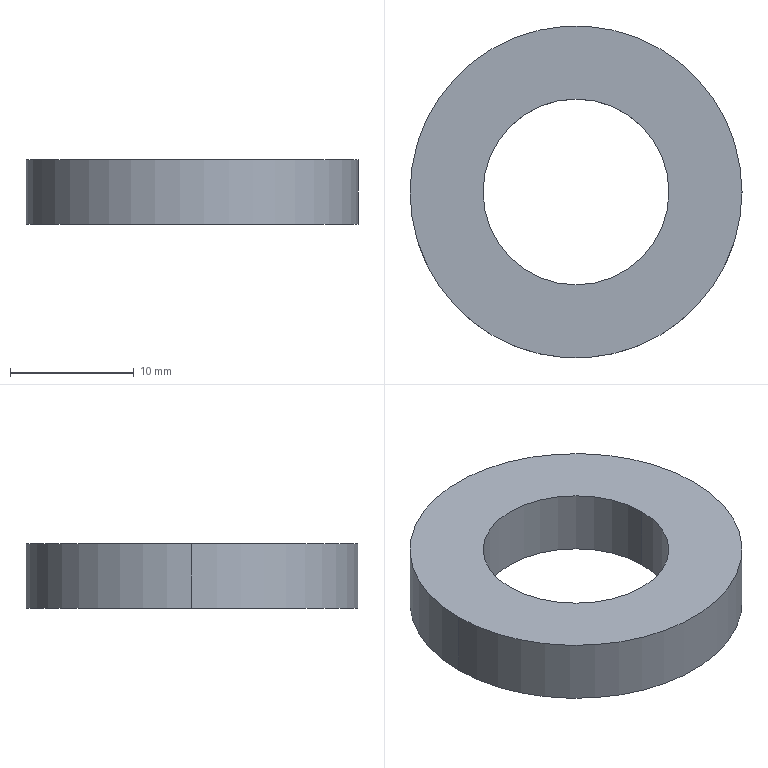Part | SolidWorks | features BaseBody 1 | 1 solid | 6 faces | box 26.799 x 26.799 x 5.237 mm | volume 2029 mm3 | cylinder 4 | plane 2 | commonest cylinder face diameters 15 x2 26.799 x2
STEP:
#1=CARTESIAN_POINT('',(17.927,0.,0.));
#2=VERTEX_POINT('',#1);
#3=CARTESIAN_POINT('',(-8.872,0.,0.));
#4=VERTEX_POINT('',#3);
#5=CARTESIAN_POINT('',(4.528,0.,0.));
#6=DIRECTION('',(0.,0.,1.));
#7=DIRECTION('',(1.,0.,0.));
#8=AXIS2_PLACEMENT_3D('',#5,#6,#7);
#9=CIRCLE('',#8,13.4);
#10=EDGE_CURVE('',#2,#4,#9,.T.);
#11=ORIENTED_EDGE('',*,*,#10,.T.);
#12=CARTESIAN_POINT('',(-8.872,0.,5.237));
#13=VERTEX_POINT('',#12);
#14=CARTESIAN_POINT('',(-8.872,0.,0.));
#15=DIRECTION('',(0.,0.,1.));
#16=VECTOR('',#15,1000.);
#17=LINE('',#14,#16);
#18=EDGE_CURVE('',#4,#13,#17,.T.);
#19=ORIENTED_EDGE('',*,*,#18,.T.);
#20=CARTESIAN_POINT('',(17.927,0.,5.237));
#21=VERTEX_POINT('',#20);
#22=CARTESIAN_POINT('',(4.528,0.,5.237));
#23=DIRECTION('',(0.,0.,-1.));
#24=DIRECTION('',(1.,0.,0.));
#25=AXIS2_PLACEMENT_3D('',#22,#23,#24);
#26=CIRCLE('',#25,13.4);
#27=EDGE_CURVE('',#13,#21,#26,.T.);
#28=ORIENTED_EDGE('',*,*,#27,.T.);
#29=CARTESIAN_POINT('',(17.927,0.,0.));
#30=DIRECTION('',(0.,0.,1.));
#31=VECTOR('',#30,1000.);
#32=LINE('',#29,#31);
#33=EDGE_CURVE('',#2,#21,#32,.T.);
#34=ORIENTED_EDGE('',*,*,#33,.F.);
#35=EDGE_LOOP('',(#11,#19,#28,#34));
#36=FACE_OUTER_BOUND('',#35,.T.);
#37=CARTESIAN_POINT('',(4.528,0.,0.));
#38=DIRECTION('',(0.,0.,1.));
#39=DIRECTION('',(1.,0.,0.));
#40=AXIS2_PLACEMENT_3D('',#37,#38,#39);
#41=CYLINDRICAL_SURFACE('',#40,13.4);
#42=ADVANCED_FACE('',(#36),#41,.T.);
#43=CARTESIAN_POINT('',(12.028,0.,0.));
#44=VERTEX_POINT('',#43);
#45=CARTESIAN_POINT('',(-2.972,0.,0.));
#46=VERTEX_POINT('',#45);
#47=CARTESIAN_POINT('',(4.528,0.,0.));
#48=DIRECTION('',(0.,0.,-1.));
#49=DIRECTION('',(1.,0.,0.));
#50=AXIS2_PLACEMENT_3D('',#47,#48,#49);
#51=CIRCLE('',#50,7.5);
#52=EDGE_CURVE('',#44,#46,#51,.T.);
#53=ORIENTED_EDGE('',*,*,#52,.T.);
#54=CARTESIAN_POINT('',(-2.972,0.,5.237));
#55=VERTEX_POINT('',#54);
#56=CARTESIAN_POINT('',(-2.972,0.,0.));
#57=DIRECTION('',(0.,0.,1.));
#58=VECTOR('',#57,1000.);
#59=LINE('',#56,#58);
#60=EDGE_CURVE('',#46,#55,#59,.T.);
#61=ORIENTED_EDGE('',*,*,#60,.T.);
#62=CARTESIAN_POINT('',(12.028,0.,5.237));
#63=VERTEX_POINT('',#62);
#64=CARTESIAN_POINT('',(4.528,0.,5.237));
#65=DIRECTION('',(0.,0.,-1.));
#66=DIRECTION('',(1.,0.,0.));
#67=AXIS2_PLACEMENT_3D('',#64,#65,#66);
#68=CIRCLE('',#67,7.5);
#69=EDGE_CURVE('',#63,#55,#68,.T.);
#70=ORIENTED_EDGE('',*,*,#69,.F.);
#71=CARTESIAN_POINT('',(12.028,0.,0.));
#72=DIRECTION('',(0.,0.,1.));
#73=VECTOR('',#72,1000.);
#74=LINE('',#71,#73);
#75=EDGE_CURVE('',#44,#63,#74,.T.);
#76=ORIENTED_EDGE('',*,*,#75,.F.);
#77=EDGE_LOOP('',(#53,#61,#70,#76));
#78=FACE_OUTER_BOUND('',#77,.T.);
#79=CARTESIAN_POINT('',(4.528,0.,0.));
#80=DIRECTION('',(0.,0.,1.));
#81=DIRECTION('',(1.,0.,0.));
#82=AXIS2_PLACEMENT_3D('',#79,#80,#81);
#83=CYLINDRICAL_SURFACE('',#82,7.5);
#84=ADVANCED_FACE('',(#78),#83,.F.);
#85=ORIENTED_EDGE('',*,*,#18,.F.);
#86=CARTESIAN_POINT('',(4.528,0.,0.));
#87=DIRECTION('',(0.,0.,1.));
#88=DIRECTION('',(1.,0.,0.));
#89=AXIS2_PLACEMENT_3D('',#86,#87,#88);
#90=CIRCLE('',#89,13.4);
#91=EDGE_CURVE('',#4,#2,#90,.T.);
#92=ORIENTED_EDGE('',*,*,#91,.T.);
#93=ORIENTED_EDGE('',*,*,#33,.T.);
#94=CARTESIAN_POINT('',(4.528,0.,5.237));
#95=DIRECTION('',(0.,0.,-1.));
#96=DIRECTION('',(1.,0.,0.));
#97=AXIS2_PLACEMENT_3D('',#94,#95,#96);
#98=CIRCLE('',#97,13.4);
#99=EDGE_CURVE('',#21,#13,#98,.T.);
#100=ORIENTED_EDGE('',*,*,#99,.T.);
#101=EDGE_LOOP('',(#85,#92,#93,#100));
#102=FACE_OUTER_BOUND('',#101,.T.);
#103=CARTESIAN_POINT('',(4.528,0.,0.));
#104=DIRECTION('',(0.,0.,1.));
#105=DIRECTION('',(1.,0.,0.));
#106=AXIS2_PLACEMENT_3D('',#103,#104,#105);
#107=CYLINDRICAL_SURFACE('',#106,13.4);
#108=ADVANCED_FACE('',(#102),#107,.T.);
#109=ORIENTED_EDGE('',*,*,#52,.F.);
#110=CARTESIAN_POINT('',(4.528,0.,0.));
#111=DIRECTION('',(0.,0.,-1.));
#112=DIRECTION('',(1.,0.,0.));
#113=AXIS2_PLACEMENT_3D('',#110,#111,#112);
#114=CIRCLE('',#113,7.5);
#115=EDGE_CURVE('',#46,#44,#114,.T.);
#116=ORIENTED_EDGE('',*,*,#115,.F.);
#117=EDGE_LOOP('',(#109,#116));
#118=FACE_BOUND('',#117,.T.);
#119=ORIENTED_EDGE('',*,*,#10,.F.);
#120=ORIENTED_EDGE('',*,*,#91,.F.);
#121=EDGE_LOOP('',(#119,#120));
#122=FACE_OUTER_BOUND('',#121,.T.);
#123=CARTESIAN_POINT('',(4.528,0.,0.));
#124=DIRECTION('',(0.,0.,1.));
#125=DIRECTION('',(1.,0.,0.));
#126=AXIS2_PLACEMENT_3D('',#123,#124,#125);
#127=PLANE('',#126);
#128=ADVANCED_FACE('',(#118,#122),#127,.F.);
#129=ORIENTED_EDGE('',*,*,#69,.T.);
#130=CARTESIAN_POINT('',(4.528,0.,5.237));
#131=DIRECTION('',(0.,0.,-1.));
#132=DIRECTION('',(1.,0.,0.));
#133=AXIS2_PLACEMENT_3D('',#130,#131,#132);
#134=CIRCLE('',#133,7.5);
#135=EDGE_CURVE('',#55,#63,#134,.T.);
#136=ORIENTED_EDGE('',*,*,#135,.T.);
#137=EDGE_LOOP('',(#129,#136));
#138=FACE_BOUND('',#137,.T.);
#139=ORIENTED_EDGE('',*,*,#99,.F.);
#140=ORIENTED_EDGE('',*,*,#27,.F.);
#141=EDGE_LOOP('',(#139,#140));
#142=FACE_OUTER_BOUND('',#141,.T.);
#143=CARTESIAN_POINT('',(4.528,0.,5.237));
#144=DIRECTION('',(0.,0.,1.));
#145=DIRECTION('',(1.,0.,0.));
#146=AXIS2_PLACEMENT_3D('',#143,#144,#145);
#147=PLANE('',#146);
#148=ADVANCED_FACE('',(#138,#142),#147,.T.);
#149=ORIENTED_EDGE('',*,*,#60,.F.);
#150=ORIENTED_EDGE('',*,*,#115,.T.);
#151=ORIENTED_EDGE('',*,*,#75,.T.);
#152=ORIENTED_EDGE('',*,*,#135,.F.);
#153=EDGE_LOOP('',(#149,#150,#151,#152));
#154=FACE_OUTER_BOUND('',#153,.T.);
#155=CARTESIAN_POINT('',(4.528,0.,0.));
#156=DIRECTION('',(0.,0.,1.));
#157=DIRECTION('',(1.,0.,0.));
#158=AXIS2_PLACEMENT_3D('',#155,#156,#157);
#159=CYLINDRICAL_SURFACE('',#158,7.5);
#160=ADVANCED_FACE('',(#154),#159,.F.);
#161=CLOSED_SHELL('',(#42,#84,#108,#128,#148,#160));
#162=MANIFOLD_SOLID_BREP('',#161);
#163=CARTESIAN_POINT('',(0.,0.,0.));
#164=DIRECTION('',(0.,0.,1.));
#165=DIRECTION('',(1.,0.,0.));
#166=AXIS2_PLACEMENT_3D('',#163,#164,#165);
#167=(LENGTH_UNIT()NAMED_UNIT(*)SI_UNIT(.MILLI.,.METRE.));
#168=UNCERTAINTY_MEASURE_WITH_UNIT(LENGTH_MEASURE(0.00001),#167,'','');
#169=(NAMED_UNIT(*)PLANE_ANGLE_UNIT()SI_UNIT($,.RADIAN.));
#170=(NAMED_UNIT(*)SI_UNIT($,.STERADIAN.)SOLID_ANGLE_UNIT());
#171=(GEOMETRIC_REPRESENTATION_CONTEXT(3)GLOBAL_UNCERTAINTY_ASSIGNED_CONTEXT((#168))GLOBAL_UNIT_ASSIGNED_CONTEXT((#167,#169,#170))REPRESENTATION_CONTEXT('',''));
#172=ADVANCED_BREP_SHAPE_REPRESENTATION('',(#162,#166),#171);